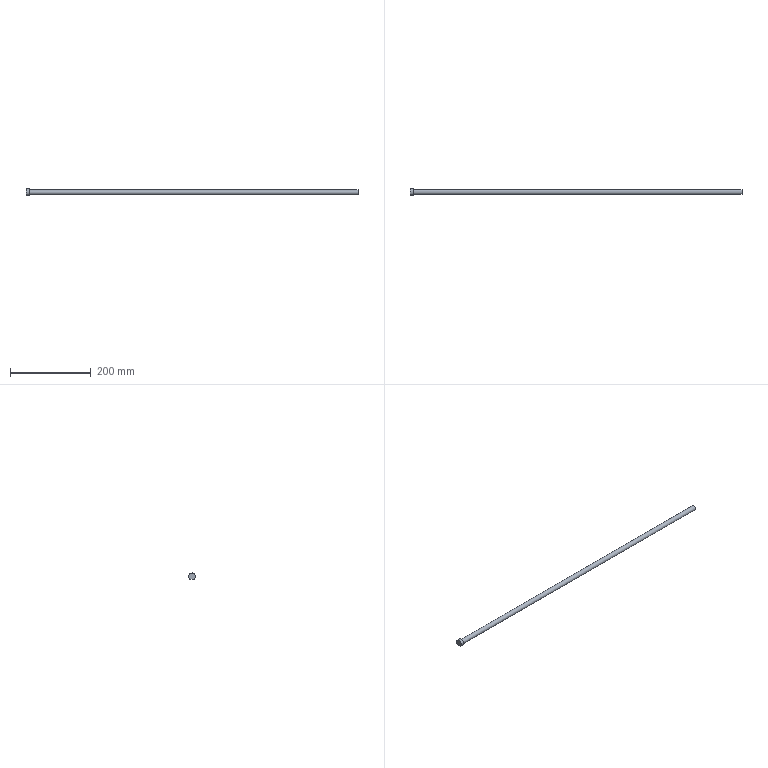Part | STEP file | solid 40 | 1 solid | 6 faces | box 820 x 17 x 15 mm | volume 93531 mm3 | plane 4 | cylinder 2 | commonest cylinder face diameters 12 x1 17 x1